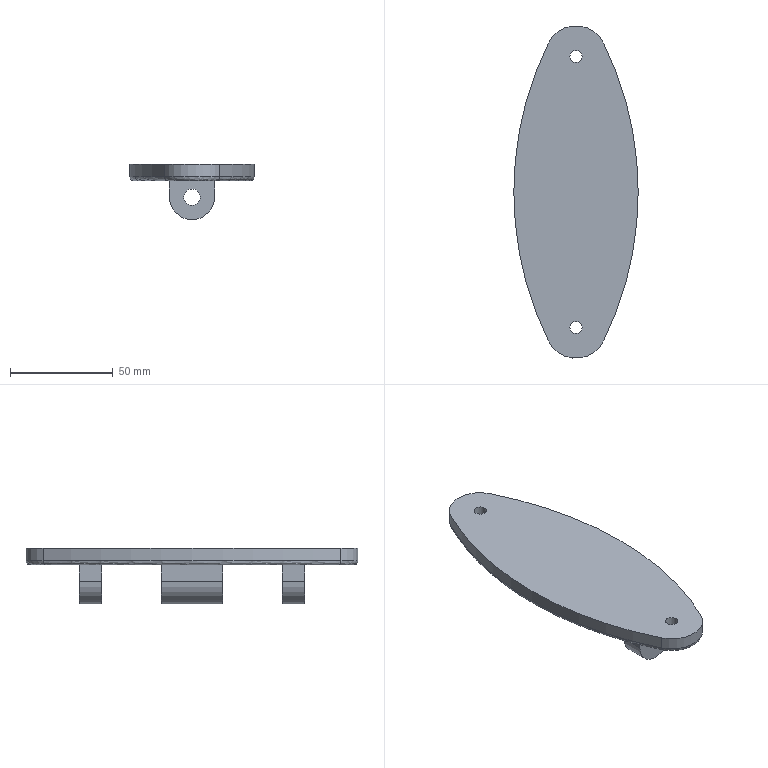Part | STEP file | 1 solid | 30 faces | box 60.601 x 162 x 27 mm | volume 75887 mm3 | plane 14 | cylinder 12 | spline 4 | commonest cylinder face diameters 8 x3 22 x3 6 x2 30 x2 330 x2